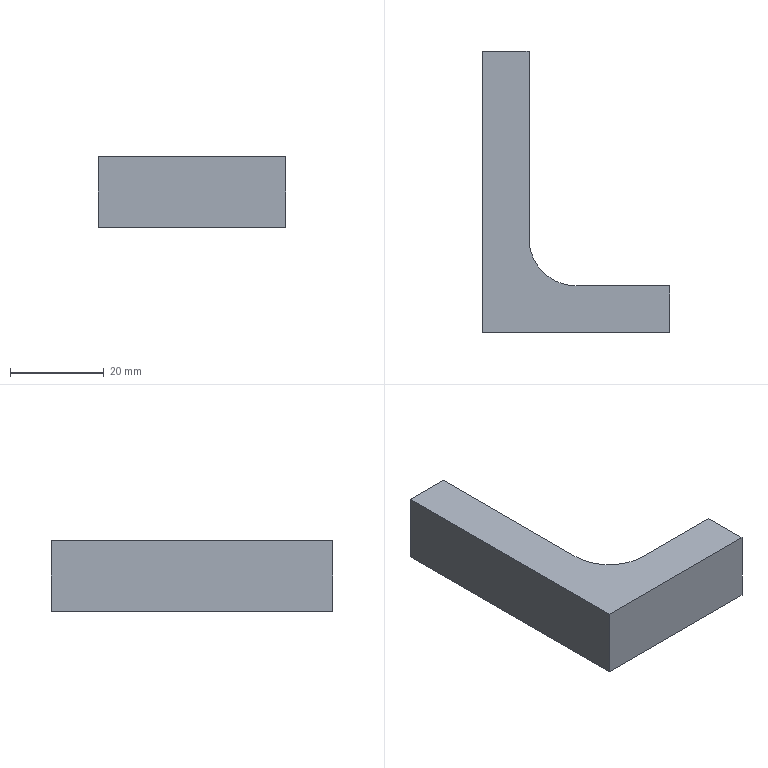Part | STEP file | 001-004-Feeding mechanism reinforcing rib | 1 solid | 9 faces | box 40 x 60 x 15 mm | volume 13822 mm3 | plane 8 | cylinder 1 | commonest cylinder face diameters 20 x1
STEP:
#1=CARTESIAN_POINT('',(0.,0.,0.));
#2=DIRECTION('',(0.,0.,1.));
#3=DIRECTION('',(1.,0.,0.));
#4=AXIS2_PLACEMENT_3D('',#1,#2,#3);
#5=CARTESIAN_POINT('',(20.,-30.,0.));
#6=VERTEX_POINT('',#5);
#7=CARTESIAN_POINT('',(20.,-20.,0.));
#8=VERTEX_POINT('',#7);
#9=CARTESIAN_POINT('',(20.,-30.,0.));
#10=DIRECTION('',(0.,1.,0.));
#11=VECTOR('',#10,1.);
#12=LINE('',#9,#11);
#13=CARTESIAN_POINT('',(20.,-30.,15.));
#14=DIRECTION('',(-1.,0.,0.));
#15=DIRECTION('',(0.,0.,1.));
#16=AXIS2_PLACEMENT_3D('',#13,#14,#15);
#17=PLANE('',#16);
#18=CARTESIAN_POINT('',(-15.,0.));
#19=DIRECTION('',(0.,1.));
#20=VECTOR('',#19,1.);
#21=LINE('',#18,#20);
#22=(GEOMETRIC_REPRESENTATION_CONTEXT(2)PARAMETRIC_REPRESENTATION_CONTEXT()REPRESENTATION_CONTEXT('',''));
#23=DEFINITIONAL_REPRESENTATION('',(#21),#22);
#24=PCURVE('',#17,#23);
#25=CARTESIAN_POINT('',(0.,0.,0.));
#26=DIRECTION('',(0.,0.,-1.));
#27=DIRECTION('',(-1.,0.,0.));
#28=AXIS2_PLACEMENT_3D('',#25,#26,#27);
#29=PLANE('',#28);
#30=CARTESIAN_POINT('',(-20.,-30.));
#31=DIRECTION('',(0.,1.));
#32=VECTOR('',#31,1.);
#33=LINE('',#30,#32);
#34=(GEOMETRIC_REPRESENTATION_CONTEXT(2)PARAMETRIC_REPRESENTATION_CONTEXT()REPRESENTATION_CONTEXT('',''));
#35=DEFINITIONAL_REPRESENTATION('',(#33),#34);
#36=PCURVE('',#29,#35);
#37=SURFACE_CURVE('',#12,(#24,#36),.PCURVE_S1.);
#38=EDGE_CURVE('',#6,#8,#37,.T.);
#39=ORIENTED_EDGE('',*,*,#38,.T.);
#40=CARTESIAN_POINT('',(20.,-20.,15.));
#41=VERTEX_POINT('',#40);
#42=CARTESIAN_POINT('',(20.,-20.,0.));
#43=DIRECTION('',(0.,0.,1.));
#44=VECTOR('',#43,1.);
#45=LINE('',#42,#44);
#46=CARTESIAN_POINT('',(-15.,10.));
#47=DIRECTION('',(1.,0.));
#48=VECTOR('',#47,1.);
#49=LINE('',#46,#48);
#50=(GEOMETRIC_REPRESENTATION_CONTEXT(2)PARAMETRIC_REPRESENTATION_CONTEXT()REPRESENTATION_CONTEXT('',''));
#51=DEFINITIONAL_REPRESENTATION('',(#49),#50);
#52=PCURVE('',#17,#51);
#53=CARTESIAN_POINT('',(20.,-20.,0.));
#54=DIRECTION('',(0.,-1.,0.));
#55=DIRECTION('',(1.,0.,0.));
#56=AXIS2_PLACEMENT_3D('',#53,#54,#55);
#57=PLANE('',#56);
#58=CARTESIAN_POINT('',(0.,0.));
#59=DIRECTION('',(0.,1.));
#60=VECTOR('',#59,1.);
#61=LINE('',#58,#60);
#62=(GEOMETRIC_REPRESENTATION_CONTEXT(2)PARAMETRIC_REPRESENTATION_CONTEXT()REPRESENTATION_CONTEXT('',''));
#63=DEFINITIONAL_REPRESENTATION('',(#61),#62);
#64=PCURVE('',#57,#63);
#65=SURFACE_CURVE('',#45,(#52,#64),.PCURVE_S1.);
#66=EDGE_CURVE('',#8,#41,#65,.T.);
#67=ORIENTED_EDGE('',*,*,#66,.T.);
#68=CARTESIAN_POINT('',(20.,-30.,15.));
#69=VERTEX_POINT('',#68);
#70=CARTESIAN_POINT('',(20.,-30.,15.));
#71=DIRECTION('',(0.,1.,0.));
#72=VECTOR('',#71,1.);
#73=LINE('',#70,#72);
#74=CARTESIAN_POINT('',(0.,0.));
#75=DIRECTION('',(0.,1.));
#76=VECTOR('',#75,1.);
#77=LINE('',#74,#76);
#78=(GEOMETRIC_REPRESENTATION_CONTEXT(2)PARAMETRIC_REPRESENTATION_CONTEXT()REPRESENTATION_CONTEXT('',''));
#79=DEFINITIONAL_REPRESENTATION('',(#77),#78);
#80=PCURVE('',#17,#79);
#81=CARTESIAN_POINT('',(0.,0.,15.));
#82=DIRECTION('',(0.,0.,-1.));
#83=DIRECTION('',(-1.,0.,0.));
#84=AXIS2_PLACEMENT_3D('',#81,#82,#83);
#85=PLANE('',#84);
#86=CARTESIAN_POINT('',(-20.,-30.));
#87=DIRECTION('',(0.,1.));
#88=VECTOR('',#87,1.);
#89=LINE('',#86,#88);
#90=(GEOMETRIC_REPRESENTATION_CONTEXT(2)PARAMETRIC_REPRESENTATION_CONTEXT()REPRESENTATION_CONTEXT('',''));
#91=DEFINITIONAL_REPRESENTATION('',(#89),#90);
#92=PCURVE('',#85,#91);
#93=SURFACE_CURVE('',#73,(#80,#92),.PCURVE_S1.);
#94=EDGE_CURVE('',#69,#41,#93,.T.);
#95=ORIENTED_EDGE('',*,*,#94,.F.);
#96=CARTESIAN_POINT('',(20.,-30.,15.));
#97=DIRECTION('',(0.,0.,-1.));
#98=VECTOR('',#97,1.);
#99=LINE('',#96,#98);
#100=CARTESIAN_POINT('',(0.,0.));
#101=DIRECTION('',(-1.,0.));
#102=VECTOR('',#101,1.);
#103=LINE('',#100,#102);
#104=(GEOMETRIC_REPRESENTATION_CONTEXT(2)PARAMETRIC_REPRESENTATION_CONTEXT()REPRESENTATION_CONTEXT('',''));
#105=DEFINITIONAL_REPRESENTATION('',(#103),#104);
#106=PCURVE('',#17,#105);
#107=CARTESIAN_POINT('',(-20.,-30.,15.));
#108=DIRECTION('',(0.,1.,0.));
#109=DIRECTION('',(0.,0.,1.));
#110=AXIS2_PLACEMENT_3D('',#107,#108,#109);
#111=PLANE('',#110);
#112=CARTESIAN_POINT('',(0.,40.));
#113=DIRECTION('',(-1.,0.));
#114=VECTOR('',#113,1.);
#115=LINE('',#112,#114);
#116=(GEOMETRIC_REPRESENTATION_CONTEXT(2)PARAMETRIC_REPRESENTATION_CONTEXT()REPRESENTATION_CONTEXT('',''));
#117=DEFINITIONAL_REPRESENTATION('',(#115),#116);
#118=PCURVE('',#111,#117);
#119=SURFACE_CURVE('',#99,(#106,#118),.PCURVE_S1.);
#120=EDGE_CURVE('',#69,#6,#119,.T.);
#121=ORIENTED_EDGE('',*,*,#120,.T.);
#122=EDGE_LOOP('',(#39,#67,#95,#121));
#123=FACE_BOUND('',#122,.T.);
#124=ADVANCED_FACE('',(#123),#17,.F.);
#125=CARTESIAN_POINT('',(-10.,30.,15.));
#126=VERTEX_POINT('',#125);
#127=CARTESIAN_POINT('',(-20.,30.,15.));
#128=VERTEX_POINT('',#127);
#129=CARTESIAN_POINT('',(-20.,30.,15.));
#130=DIRECTION('',(-1.,0.,0.));
#131=VECTOR('',#130,1.);
#132=LINE('',#129,#131);
#133=CARTESIAN_POINT('',(-20.,30.,15.));
#134=DIRECTION('',(0.,-1.,0.));
#135=DIRECTION('',(0.,0.,-1.));
#136=AXIS2_PLACEMENT_3D('',#133,#134,#135);
#137=PLANE('',#136);
#138=CARTESIAN_POINT('',(0.,0.));
#139=DIRECTION('',(0.,-1.));
#140=VECTOR('',#139,1.);
#141=LINE('',#138,#140);
#142=(GEOMETRIC_REPRESENTATION_CONTEXT(2)PARAMETRIC_REPRESENTATION_CONTEXT()REPRESENTATION_CONTEXT('',''));
#143=DEFINITIONAL_REPRESENTATION('',(#141),#142);
#144=PCURVE('',#137,#143);
#145=CARTESIAN_POINT('',(20.,30.));
#146=DIRECTION('',(1.,0.));
#147=VECTOR('',#146,1.);
#148=LINE('',#145,#147);
#149=(GEOMETRIC_REPRESENTATION_CONTEXT(2)PARAMETRIC_REPRESENTATION_CONTEXT()REPRESENTATION_CONTEXT('',''));
#150=DEFINITIONAL_REPRESENTATION('',(#148),#149);
#151=PCURVE('',#85,#150);
#152=SURFACE_CURVE('',#132,(#144,#151),.PCURVE_S1.);
#153=EDGE_CURVE('',#126,#128,#152,.T.);
#154=ORIENTED_EDGE('',*,*,#153,.F.);
#155=CARTESIAN_POINT('',(-10.,30.,0.));
#156=VERTEX_POINT('',#155);
#157=CARTESIAN_POINT('',(-10.,30.,0.));
#158=DIRECTION('',(0.,0.,1.));
#159=VECTOR('',#158,1.);
#160=LINE('',#157,#159);
#161=CARTESIAN_POINT('',(15.,10.));
#162=DIRECTION('',(-1.,0.));
#163=VECTOR('',#162,1.);
#164=LINE('',#161,#163);
#165=(GEOMETRIC_REPRESENTATION_CONTEXT(2)PARAMETRIC_REPRESENTATION_CONTEXT()REPRESENTATION_CONTEXT('',''));
#166=DEFINITIONAL_REPRESENTATION('',(#164),#165);
#167=PCURVE('',#137,#166);
#168=CARTESIAN_POINT('',(-10.,30.,0.));
#169=DIRECTION('',(-1.,0.,0.));
#170=DIRECTION('',(0.,-1.,0.));
#171=AXIS2_PLACEMENT_3D('',#168,#169,#170);
#172=PLANE('',#171);
#173=CARTESIAN_POINT('',(0.,0.));
#174=DIRECTION('',(0.,1.));
#175=VECTOR('',#174,1.);
#176=LINE('',#173,#175);
#177=(GEOMETRIC_REPRESENTATION_CONTEXT(2)PARAMETRIC_REPRESENTATION_CONTEXT()REPRESENTATION_CONTEXT('',''));
#178=DEFINITIONAL_REPRESENTATION('',(#176),#177);
#179=PCURVE('',#172,#178);
#180=SURFACE_CURVE('',#160,(#167,#179),.PCURVE_S1.);
#181=EDGE_CURVE('',#156,#126,#180,.T.);
#182=ORIENTED_EDGE('',*,*,#181,.F.);
#183=CARTESIAN_POINT('',(-20.,30.,0.));
#184=VERTEX_POINT('',#183);
#185=CARTESIAN_POINT('',(-20.,30.,0.));
#186=DIRECTION('',(-1.,0.,0.));
#187=VECTOR('',#186,1.);
#188=LINE('',#185,#187);
#189=CARTESIAN_POINT('',(15.,0.));
#190=DIRECTION('',(0.,-1.));
#191=VECTOR('',#190,1.);
#192=LINE('',#189,#191);
#193=(GEOMETRIC_REPRESENTATION_CONTEXT(2)PARAMETRIC_REPRESENTATION_CONTEXT()REPRESENTATION_CONTEXT('',''));
#194=DEFINITIONAL_REPRESENTATION('',(#192),#193);
#195=PCURVE('',#137,#194);
#196=CARTESIAN_POINT('',(20.,30.));
#197=DIRECTION('',(1.,0.));
#198=VECTOR('',#197,1.);
#199=LINE('',#196,#198);
#200=(GEOMETRIC_REPRESENTATION_CONTEXT(2)PARAMETRIC_REPRESENTATION_CONTEXT()REPRESENTATION_CONTEXT('',''));
#201=DEFINITIONAL_REPRESENTATION('',(#199),#200);
#202=PCURVE('',#29,#201);
#203=SURFACE_CURVE('',#188,(#195,#202),.PCURVE_S1.);
#204=EDGE_CURVE('',#156,#184,#203,.T.);
#205=ORIENTED_EDGE('',*,*,#204,.T.);
#206=CARTESIAN_POINT('',(-20.,30.,15.));
#207=DIRECTION('',(0.,0.,-1.));
#208=VECTOR('',#207,1.);
#209=LINE('',#206,#208);
#210=CARTESIAN_POINT('',(0.,0.));
#211=DIRECTION('',(1.,0.));
#212=VECTOR('',#211,1.);
#213=LINE('',#210,#212);
#214=(GEOMETRIC_REPRESENTATION_CONTEXT(2)PARAMETRIC_REPRESENTATION_CONTEXT()REPRESENTATION_CONTEXT('',''));
#215=DEFINITIONAL_REPRESENTATION('',(#213),#214);
#216=PCURVE('',#137,#215);
#217=CARTESIAN_POINT('',(-20.,-30.,15.));
#218=DIRECTION('',(1.,0.,0.));
#219=DIRECTION('',(0.,0.,-1.));
#220=AXIS2_PLACEMENT_3D('',#217,#218,#219);
#221=PLANE('',#220);
#222=CARTESIAN_POINT('',(0.,60.));
#223=DIRECTION('',(1.,0.));
#224=VECTOR('',#223,1.);
#225=LINE('',#222,#224);
#226=(GEOMETRIC_REPRESENTATION_CONTEXT(2)PARAMETRIC_REPRESENTATION_CONTEXT()REPRESENTATION_CONTEXT('',''));
#227=DEFINITIONAL_REPRESENTATION('',(#225),#226);
#228=PCURVE('',#221,#227);
#229=SURFACE_CURVE('',#209,(#216,#228),.PCURVE_S1.);
#230=EDGE_CURVE('',#128,#184,#229,.T.);
#231=ORIENTED_EDGE('',*,*,#230,.F.);
#232=EDGE_LOOP('',(#154,#182,#205,#231));
#233=FACE_BOUND('',#232,.T.);
#234=ADVANCED_FACE('',(#233),#137,.F.);
#235=CARTESIAN_POINT('',(-20.,-30.,0.));
#236=VERTEX_POINT('',#235);
#237=CARTESIAN_POINT('',(-20.,-30.,0.));
#238=DIRECTION('',(0.,-1.,0.));
#239=VECTOR('',#238,1.);
#240=LINE('',#237,#239);
#241=CARTESIAN_POINT('',(15.,0.));
#242=DIRECTION('',(0.,-1.));
#243=VECTOR('',#242,1.);
#244=LINE('',#241,#243);
#245=(GEOMETRIC_REPRESENTATION_CONTEXT(2)PARAMETRIC_REPRESENTATION_CONTEXT()REPRESENTATION_CONTEXT('',''));
#246=DEFINITIONAL_REPRESENTATION('',(#244),#245);
#247=PCURVE('',#221,#246);
#248=CARTESIAN_POINT('',(20.,-30.));
#249=DIRECTION('',(0.,-1.));
#250=VECTOR('',#249,1.);
#251=LINE('',#248,#250);
#252=(GEOMETRIC_REPRESENTATION_CONTEXT(2)PARAMETRIC_REPRESENTATION_CONTEXT()REPRESENTATION_CONTEXT('',''));
#253=DEFINITIONAL_REPRESENTATION('',(#251),#252);
#254=PCURVE('',#29,#253);
#255=SURFACE_CURVE('',#240,(#247,#254),.PCURVE_S1.);
#256=EDGE_CURVE('',#184,#236,#255,.T.);
#257=ORIENTED_EDGE('',*,*,#256,.T.);
#258=CARTESIAN_POINT('',(-20.,-30.,15.));
#259=VERTEX_POINT('',#258);
#260=CARTESIAN_POINT('',(-20.,-30.,15.));
#261=DIRECTION('',(0.,0.,-1.));
#262=VECTOR('',#261,1.);
#263=LINE('',#260,#262);
#264=CARTESIAN_POINT('',(0.,0.));
#265=DIRECTION('',(1.,0.));
#266=VECTOR('',#265,1.);
#267=LINE('',#264,#266);
#268=(GEOMETRIC_REPRESENTATION_CONTEXT(2)PARAMETRIC_REPRESENTATION_CONTEXT()REPRESENTATION_CONTEXT('',''));
#269=DEFINITIONAL_REPRESENTATION('',(#267),#268);
#270=PCURVE('',#221,#269);
#271=CARTESIAN_POINT('',(0.,0.));
#272=DIRECTION('',(-1.,0.));
#273=VECTOR('',#272,1.);
#274=LINE('',#271,#273);
#275=(GEOMETRIC_REPRESENTATION_CONTEXT(2)PARAMETRIC_REPRESENTATION_CONTEXT()REPRESENTATION_CONTEXT('',''));
#276=DEFINITIONAL_REPRESENTATION('',(#274),#275);
#277=PCURVE('',#111,#276);
#278=SURFACE_CURVE('',#263,(#270,#277),.PCURVE_S1.);
#279=EDGE_CURVE('',#259,#236,#278,.T.);
#280=ORIENTED_EDGE('',*,*,#279,.F.);
#281=CARTESIAN_POINT('',(-20.,-30.,15.));
#282=DIRECTION('',(0.,-1.,0.));
#283=VECTOR('',#282,1.);
#284=LINE('',#281,#283);
#285=CARTESIAN_POINT('',(0.,0.));
#286=DIRECTION('',(0.,-1.));
#287=VECTOR('',#286,1.);
#288=LINE('',#285,#287);
#289=(GEOMETRIC_REPRESENTATION_CONTEXT(2)PARAMETRIC_REPRESENTATION_CONTEXT()REPRESENTATION_CONTEXT('',''));
#290=DEFINITIONAL_REPRESENTATION('',(#288),#289);
#291=PCURVE('',#221,#290);
#292=CARTESIAN_POINT('',(20.,-30.));
#293=DIRECTION('',(0.,-1.));
#294=VECTOR('',#293,1.);
#295=LINE('',#292,#294);
#296=(GEOMETRIC_REPRESENTATION_CONTEXT(2)PARAMETRIC_REPRESENTATION_CONTEXT()REPRESENTATION_CONTEXT('',''));
#297=DEFINITIONAL_REPRESENTATION('',(#295),#296);
#298=PCURVE('',#85,#297);
#299=SURFACE_CURVE('',#284,(#291,#298),.PCURVE_S1.);
#300=EDGE_CURVE('',#128,#259,#299,.T.);
#301=ORIENTED_EDGE('',*,*,#300,.F.);
#302=ORIENTED_EDGE('',*,*,#230,.T.);
#303=EDGE_LOOP('',(#257,#280,#301,#302));
#304=FACE_BOUND('',#303,.T.);
#305=ADVANCED_FACE('',(#304),#221,.F.);
#306=CARTESIAN_POINT('',(-20.,-30.,0.));
#307=DIRECTION('',(1.,0.,0.));
#308=VECTOR('',#307,1.);
#309=LINE('',#306,#308);
#310=CARTESIAN_POINT('',(-15.,0.));
#311=DIRECTION('',(0.,1.));
#312=VECTOR('',#311,1.);
#313=LINE('',#310,#312);
#314=(GEOMETRIC_REPRESENTATION_CONTEXT(2)PARAMETRIC_REPRESENTATION_CONTEXT()REPRESENTATION_CONTEXT('',''));
#315=DEFINITIONAL_REPRESENTATION('',(#313),#314);
#316=PCURVE('',#111,#315);
#317=CARTESIAN_POINT('',(20.,-30.));
#318=DIRECTION('',(-1.,0.));
#319=VECTOR('',#318,1.);
#320=LINE('',#317,#319);
#321=(GEOMETRIC_REPRESENTATION_CONTEXT(2)PARAMETRIC_REPRESENTATION_CONTEXT()REPRESENTATION_CONTEXT('',''));
#322=DEFINITIONAL_REPRESENTATION('',(#320),#321);
#323=PCURVE('',#29,#322);
#324=SURFACE_CURVE('',#309,(#316,#323),.PCURVE_S1.);
#325=EDGE_CURVE('',#236,#6,#324,.T.);
#326=ORIENTED_EDGE('',*,*,#325,.T.);
#327=ORIENTED_EDGE('',*,*,#120,.F.);
#328=CARTESIAN_POINT('',(-20.,-30.,15.));
#329=DIRECTION('',(1.,0.,0.));
#330=VECTOR('',#329,1.);
#331=LINE('',#328,#330);
#332=CARTESIAN_POINT('',(0.,0.));
#333=DIRECTION('',(0.,1.));
#334=VECTOR('',#333,1.);
#335=LINE('',#332,#334);
#336=(GEOMETRIC_REPRESENTATION_CONTEXT(2)PARAMETRIC_REPRESENTATION_CONTEXT()REPRESENTATION_CONTEXT('',''));
#337=DEFINITIONAL_REPRESENTATION('',(#335),#336);
#338=PCURVE('',#111,#337);
#339=CARTESIAN_POINT('',(20.,-30.));
#340=DIRECTION('',(-1.,0.));
#341=VECTOR('',#340,1.);
#342=LINE('',#339,#341);
#343=(GEOMETRIC_REPRESENTATION_CONTEXT(2)PARAMETRIC_REPRESENTATION_CONTEXT()REPRESENTATION_CONTEXT('',''));
#344=DEFINITIONAL_REPRESENTATION('',(#342),#343);
#345=PCURVE('',#85,#344);
#346=SURFACE_CURVE('',#331,(#338,#345),.PCURVE_S1.);
#347=EDGE_CURVE('',#259,#69,#346,.T.);
#348=ORIENTED_EDGE('',*,*,#347,.F.);
#349=ORIENTED_EDGE('',*,*,#279,.T.);
#350=EDGE_LOOP('',(#326,#327,#348,#349));
#351=FACE_BOUND('',#350,.T.);
#352=ADVANCED_FACE('',(#351),#111,.F.);
#353=ORIENTED_EDGE('',*,*,#94,.T.);
#354=CARTESIAN_POINT('',(0.,-20.,15.));
#355=VERTEX_POINT('',#354);
#356=CARTESIAN_POINT('',(20.,-20.,15.));
#357=DIRECTION('',(1.,0.,0.));
#358=VECTOR('',#357,1.);
#359=LINE('',#356,#358);
#360=CARTESIAN_POINT('',(-20.,-20.));
#361=DIRECTION('',(-1.,0.));
#362=VECTOR('',#361,1.);
#363=LINE('',#360,#362);
#364=(GEOMETRIC_REPRESENTATION_CONTEXT(2)PARAMETRIC_REPRESENTATION_CONTEXT()REPRESENTATION_CONTEXT('',''));
#365=DEFINITIONAL_REPRESENTATION('',(#363),#364);
#366=PCURVE('',#85,#365);
#367=CARTESIAN_POINT('',(0.,15.));
#368=DIRECTION('',(1.,0.));
#369=VECTOR('',#368,1.);
#370=LINE('',#367,#369);
#371=(GEOMETRIC_REPRESENTATION_CONTEXT(2)PARAMETRIC_REPRESENTATION_CONTEXT()REPRESENTATION_CONTEXT('',''));
#372=DEFINITIONAL_REPRESENTATION('',(#370),#371);
#373=PCURVE('',#57,#372);
#374=SURFACE_CURVE('',#359,(#366,#373),.PCURVE_S1.);
#375=EDGE_CURVE('',#355,#41,#374,.T.);
#376=ORIENTED_EDGE('',*,*,#375,.F.);
#377=CARTESIAN_POINT('',(-10.,-10.,15.));
#378=VERTEX_POINT('',#377);
#379=CARTESIAN_POINT('',(0.,-10.,15.));
#380=DIRECTION('',(0.,0.,-1.));
#381=DIRECTION('',(-1.,0.,0.));
#382=AXIS2_PLACEMENT_3D('',#379,#380,#381);
#383=CIRCLE('',#382,10.);
#384=CARTESIAN_POINT('',(0.,-10.));
#385=DIRECTION('',(1.,0.));
#386=AXIS2_PLACEMENT_2D('',#384,#385);
#387=CIRCLE('',#386,10.);
#388=(GEOMETRIC_REPRESENTATION_CONTEXT(2)PARAMETRIC_REPRESENTATION_CONTEXT()REPRESENTATION_CONTEXT('',''));
#389=DEFINITIONAL_REPRESENTATION('',(#387),#388);
#390=PCURVE('',#85,#389);
#391=CARTESIAN_POINT('',(0.,-10.,0.));
#392=DIRECTION('',(0.,0.,-1.));
#393=DIRECTION('',(-1.,0.,0.));
#394=AXIS2_PLACEMENT_3D('',#391,#392,#393);
#395=CYLINDRICAL_SURFACE('',#394,10.);
#396=CARTESIAN_POINT('',(0.,-15.));
#397=DIRECTION('',(1.,0.));
#398=VECTOR('',#397,1.);
#399=LINE('',#396,#398);
#400=(GEOMETRIC_REPRESENTATION_CONTEXT(2)PARAMETRIC_REPRESENTATION_CONTEXT()REPRESENTATION_CONTEXT('',''));
#401=DEFINITIONAL_REPRESENTATION('',(#399),#400);
#402=PCURVE('',#395,#401);
#403=SURFACE_CURVE('',#383,(#390,#402),.PCURVE_S1.);
#404=EDGE_CURVE('',#355,#378,#403,.T.);
#405=ORIENTED_EDGE('',*,*,#404,.T.);
#406=CARTESIAN_POINT('',(-10.,30.,15.));
#407=DIRECTION('',(0.,-1.,0.));
#408=VECTOR('',#407,1.);
#409=LINE('',#406,#408);
#410=CARTESIAN_POINT('',(10.,30.));
#411=DIRECTION('',(0.,-1.));
#412=VECTOR('',#411,1.);
#413=LINE('',#410,#412);
#414=(GEOMETRIC_REPRESENTATION_CONTEXT(2)PARAMETRIC_REPRESENTATION_CONTEXT()REPRESENTATION_CONTEXT('',''));
#415=DEFINITIONAL_REPRESENTATION('',(#413),#414);
#416=PCURVE('',#85,#415);
#417=CARTESIAN_POINT('',(0.,15.));
#418=DIRECTION('',(1.,0.));
#419=VECTOR('',#418,1.);
#420=LINE('',#417,#419);
#421=(GEOMETRIC_REPRESENTATION_CONTEXT(2)PARAMETRIC_REPRESENTATION_CONTEXT()REPRESENTATION_CONTEXT('',''));
#422=DEFINITIONAL_REPRESENTATION('',(#420),#421);
#423=PCURVE('',#172,#422);
#424=SURFACE_CURVE('',#409,(#416,#423),.PCURVE_S1.);
#425=EDGE_CURVE('',#126,#378,#424,.T.);
#426=ORIENTED_EDGE('',*,*,#425,.F.);
#427=ORIENTED_EDGE('',*,*,#153,.T.);
#428=ORIENTED_EDGE('',*,*,#300,.T.);
#429=ORIENTED_EDGE('',*,*,#347,.T.);
#430=EDGE_LOOP('',(#353,#376,#405,#426,#427,#428,#429));
#431=FACE_BOUND('',#430,.T.);
#432=ADVANCED_FACE('',(#431),#85,.F.);
#433=CARTESIAN_POINT('',(-10.,-10.,0.));
#434=VERTEX_POINT('',#433);
#435=CARTESIAN_POINT('',(-10.,30.,0.));
#436=DIRECTION('',(0.,-1.,0.));
#437=VECTOR('',#436,1.);
#438=LINE('',#435,#437);
#439=CARTESIAN_POINT('',(10.,30.));
#440=DIRECTION('',(0.,-1.));
#441=VECTOR('',#440,1.);
#442=LINE('',#439,#441);
#443=(GEOMETRIC_REPRESENTATION_CONTEXT(2)PARAMETRIC_REPRESENTATION_CONTEXT()REPRESENTATION_CONTEXT('',''));
#444=DEFINITIONAL_REPRESENTATION('',(#442),#443);
#445=PCURVE('',#29,#444);
#446=CARTESIAN_POINT('',(0.,0.));
#447=DIRECTION('',(1.,0.));
#448=VECTOR('',#447,1.);
#449=LINE('',#446,#448);
#450=(GEOMETRIC_REPRESENTATION_CONTEXT(2)PARAMETRIC_REPRESENTATION_CONTEXT()REPRESENTATION_CONTEXT('',''));
#451=DEFINITIONAL_REPRESENTATION('',(#449),#450);
#452=PCURVE('',#172,#451);
#453=SURFACE_CURVE('',#438,(#445,#452),.PCURVE_S1.);
#454=EDGE_CURVE('',#156,#434,#453,.T.);
#455=ORIENTED_EDGE('',*,*,#454,.T.);
#456=CARTESIAN_POINT('',(0.,-20.,0.));
#457=VERTEX_POINT('',#456);
#458=CARTESIAN_POINT('',(0.,-10.,0.));
#459=DIRECTION('',(0.,0.,1.));
#460=DIRECTION('',(-1.,0.,0.));
#461=AXIS2_PLACEMENT_3D('',#458,#459,#460);
#462=CIRCLE('',#461,10.);
#463=CARTESIAN_POINT('',(10.,-10.));
#464=CARTESIAN_POINT('',(10.,-27.321));
#465=CARTESIAN_POINT('',(-5.,-18.66));
#466=CARTESIAN_POINT('',(-20.,-10.));
#467=CARTESIAN_POINT('',(-5.,-1.34));
#468=CARTESIAN_POINT('',(10.,7.321));
#469=CARTESIAN_POINT('',(10.,-10.));
#470=(BOUNDED_CURVE()B_SPLINE_CURVE(2,(#463,#464,#465,#466,#467,#468,#469),.UNSPECIFIED.,.T.,.F.)B_SPLINE_CURVE_WITH_KNOTS((1,2,2,2,2,1),(-2.094,0.,2.094,4.189,6.283,8.378),.UNSPECIFIED.)CURVE()GEOMETRIC_REPRESENTATION_ITEM()RATIONAL_B_SPLINE_CURVE((1.,0.5,1.,0.5,1.,0.5,1.))REPRESENTATION_ITEM(''));
#471=(GEOMETRIC_REPRESENTATION_CONTEXT(2)PARAMETRIC_REPRESENTATION_CONTEXT()REPRESENTATION_CONTEXT('',''));
#472=DEFINITIONAL_REPRESENTATION('',(#470),#471);
#473=PCURVE('',#29,#472);
#474=CARTESIAN_POINT('',(6.283,0.));
#475=DIRECTION('',(-1.,0.));
#476=VECTOR('',#475,1.);
#477=LINE('',#474,#476);
#478=(GEOMETRIC_REPRESENTATION_CONTEXT(2)PARAMETRIC_REPRESENTATION_CONTEXT()REPRESENTATION_CONTEXT('',''));
#479=DEFINITIONAL_REPRESENTATION('',(#477),#478);
#480=PCURVE('',#395,#479);
#481=SURFACE_CURVE('',#462,(#473,#480),.PCURVE_S1.);
#482=EDGE_CURVE('',#434,#457,#481,.T.);
#483=ORIENTED_EDGE('',*,*,#482,.T.);
#484=CARTESIAN_POINT('',(20.,-20.,0.));
#485=DIRECTION('',(1.,0.,0.));
#486=VECTOR('',#485,1.);
#487=LINE('',#484,#486);
#488=CARTESIAN_POINT('',(-20.,-20.));
#489=DIRECTION('',(-1.,0.));
#490=VECTOR('',#489,1.);
#491=LINE('',#488,#490);
#492=(GEOMETRIC_REPRESENTATION_CONTEXT(2)PARAMETRIC_REPRESENTATION_CONTEXT()REPRESENTATION_CONTEXT('',''));
#493=DEFINITIONAL_REPRESENTATION('',(#491),#492);
#494=PCURVE('',#29,#493);
#495=CARTESIAN_POINT('',(0.,0.));
#496=DIRECTION('',(1.,0.));
#497=VECTOR('',#496,1.);
#498=LINE('',#495,#497);
#499=(GEOMETRIC_REPRESENTATION_CONTEXT(2)PARAMETRIC_REPRESENTATION_CONTEXT()REPRESENTATION_CONTEXT('',''));
#500=DEFINITIONAL_REPRESENTATION('',(#498),#499);
#501=PCURVE('',#57,#500);
#502=SURFACE_CURVE('',#487,(#494,#501),.PCURVE_S1.);
#503=EDGE_CURVE('',#457,#8,#502,.T.);
#504=ORIENTED_EDGE('',*,*,#503,.T.);
#505=ORIENTED_EDGE('',*,*,#38,.F.);
#506=ORIENTED_EDGE('',*,*,#325,.F.);
#507=ORIENTED_EDGE('',*,*,#256,.F.);
#508=ORIENTED_EDGE('',*,*,#204,.F.);
#509=EDGE_LOOP('',(#455,#483,#504,#505,#506,#507,#508));
#510=FACE_BOUND('',#509,.T.);
#511=ADVANCED_FACE('',(#510),#29,.T.);
#512=ORIENTED_EDGE('',*,*,#503,.F.);
#513=CARTESIAN_POINT('',(0.,-20.,15.));
#514=DIRECTION('',(0.,0.,1.));
#515=VECTOR('',#514,1.);
#516=LINE('',#513,#515);
#517=CARTESIAN_POINT('',(-20.,15.));
#518=DIRECTION('',(0.,1.));
#519=VECTOR('',#518,1.);
#520=LINE('',#517,#519);
#521=(GEOMETRIC_REPRESENTATION_CONTEXT(2)PARAMETRIC_REPRESENTATION_CONTEXT()REPRESENTATION_CONTEXT('',''));
#522=DEFINITIONAL_REPRESENTATION('',(#520),#521);
#523=PCURVE('',#57,#522);
#524=CARTESIAN_POINT('',(4.712,-15.));
#525=DIRECTION('',(0.,-1.));
#526=VECTOR('',#525,1.);
#527=LINE('',#524,#526);
#528=(GEOMETRIC_REPRESENTATION_CONTEXT(2)PARAMETRIC_REPRESENTATION_CONTEXT()REPRESENTATION_CONTEXT('',''));
#529=DEFINITIONAL_REPRESENTATION('',(#527),#528);
#530=PCURVE('',#395,#529);
#531=SURFACE_CURVE('',#516,(#523,#530),.PCURVE_S1.);
#532=EDGE_CURVE('',#457,#355,#531,.T.);
#533=ORIENTED_EDGE('',*,*,#532,.T.);
#534=ORIENTED_EDGE('',*,*,#375,.T.);
#535=ORIENTED_EDGE('',*,*,#66,.F.);
#536=EDGE_LOOP('',(#512,#533,#534,#535));
#537=FACE_BOUND('',#536,.T.);
#538=ADVANCED_FACE('',(#537),#57,.F.);
#539=ORIENTED_EDGE('',*,*,#425,.T.);
#540=CARTESIAN_POINT('',(-10.,-10.,0.));
#541=DIRECTION('',(0.,0.,-1.));
#542=VECTOR('',#541,1.);
#543=LINE('',#540,#542);
#544=CARTESIAN_POINT('',(40.,0.));
#545=DIRECTION('',(0.,-1.));
#546=VECTOR('',#545,1.);
#547=LINE('',#544,#546);
#548=(GEOMETRIC_REPRESENTATION_CONTEXT(2)PARAMETRIC_REPRESENTATION_CONTEXT()REPRESENTATION_CONTEXT('',''));
#549=DEFINITIONAL_REPRESENTATION('',(#547),#548);
#550=PCURVE('',#172,#549);
#551=CARTESIAN_POINT('',(6.283,0.));
#552=DIRECTION('',(0.,1.));
#553=VECTOR('',#552,1.);
#554=LINE('',#551,#553);
#555=(GEOMETRIC_REPRESENTATION_CONTEXT(2)PARAMETRIC_REPRESENTATION_CONTEXT()REPRESENTATION_CONTEXT('',''));
#556=DEFINITIONAL_REPRESENTATION('',(#554),#555);
#557=PCURVE('',#395,#556);
#558=SURFACE_CURVE('',#543,(#550,#557),.PCURVE_S1.);
#559=EDGE_CURVE('',#378,#434,#558,.T.);
#560=ORIENTED_EDGE('',*,*,#559,.T.);
#561=ORIENTED_EDGE('',*,*,#454,.F.);
#562=ORIENTED_EDGE('',*,*,#181,.T.);
#563=EDGE_LOOP('',(#539,#560,#561,#562));
#564=FACE_BOUND('',#563,.T.);
#565=ADVANCED_FACE('',(#564),#172,.F.);
#566=ORIENTED_EDGE('',*,*,#532,.T.);
#567=ORIENTED_EDGE('',*,*,#404,.T.);
#568=ORIENTED_EDGE('',*,*,#559,.T.);
#569=ORIENTED_EDGE('',*,*,#482,.T.);
#570=EDGE_LOOP('',(#566,#567,#568,#569));
#571=FACE_BOUND('',#570,.F.);
#572=ADVANCED_FACE('',(#571),#395,.F.);
#573=CLOSED_SHELL('',(#124,#234,#305,#352,#432,#511,#538,#565,#572));
#574=MANIFOLD_SOLID_BREP('',#573);
#575=(LENGTH_UNIT()NAMED_UNIT(*)SI_UNIT(.MILLI.,.METRE.));
#576=UNCERTAINTY_MEASURE_WITH_UNIT(LENGTH_MEASURE(0.0000001),#575,'','');
#577=(NAMED_UNIT(*)PLANE_ANGLE_UNIT()SI_UNIT($,.RADIAN.));
#578=(NAMED_UNIT(*)SI_UNIT($,.STERADIAN.)SOLID_ANGLE_UNIT());
#579=(GEOMETRIC_REPRESENTATION_CONTEXT(3)GLOBAL_UNCERTAINTY_ASSIGNED_CONTEXT((#576))GLOBAL_UNIT_ASSIGNED_CONTEXT((#575,#577,#578))REPRESENTATION_CONTEXT('',''));
#580=ADVANCED_BREP_SHAPE_REPRESENTATION('',(#4,#574),#579);